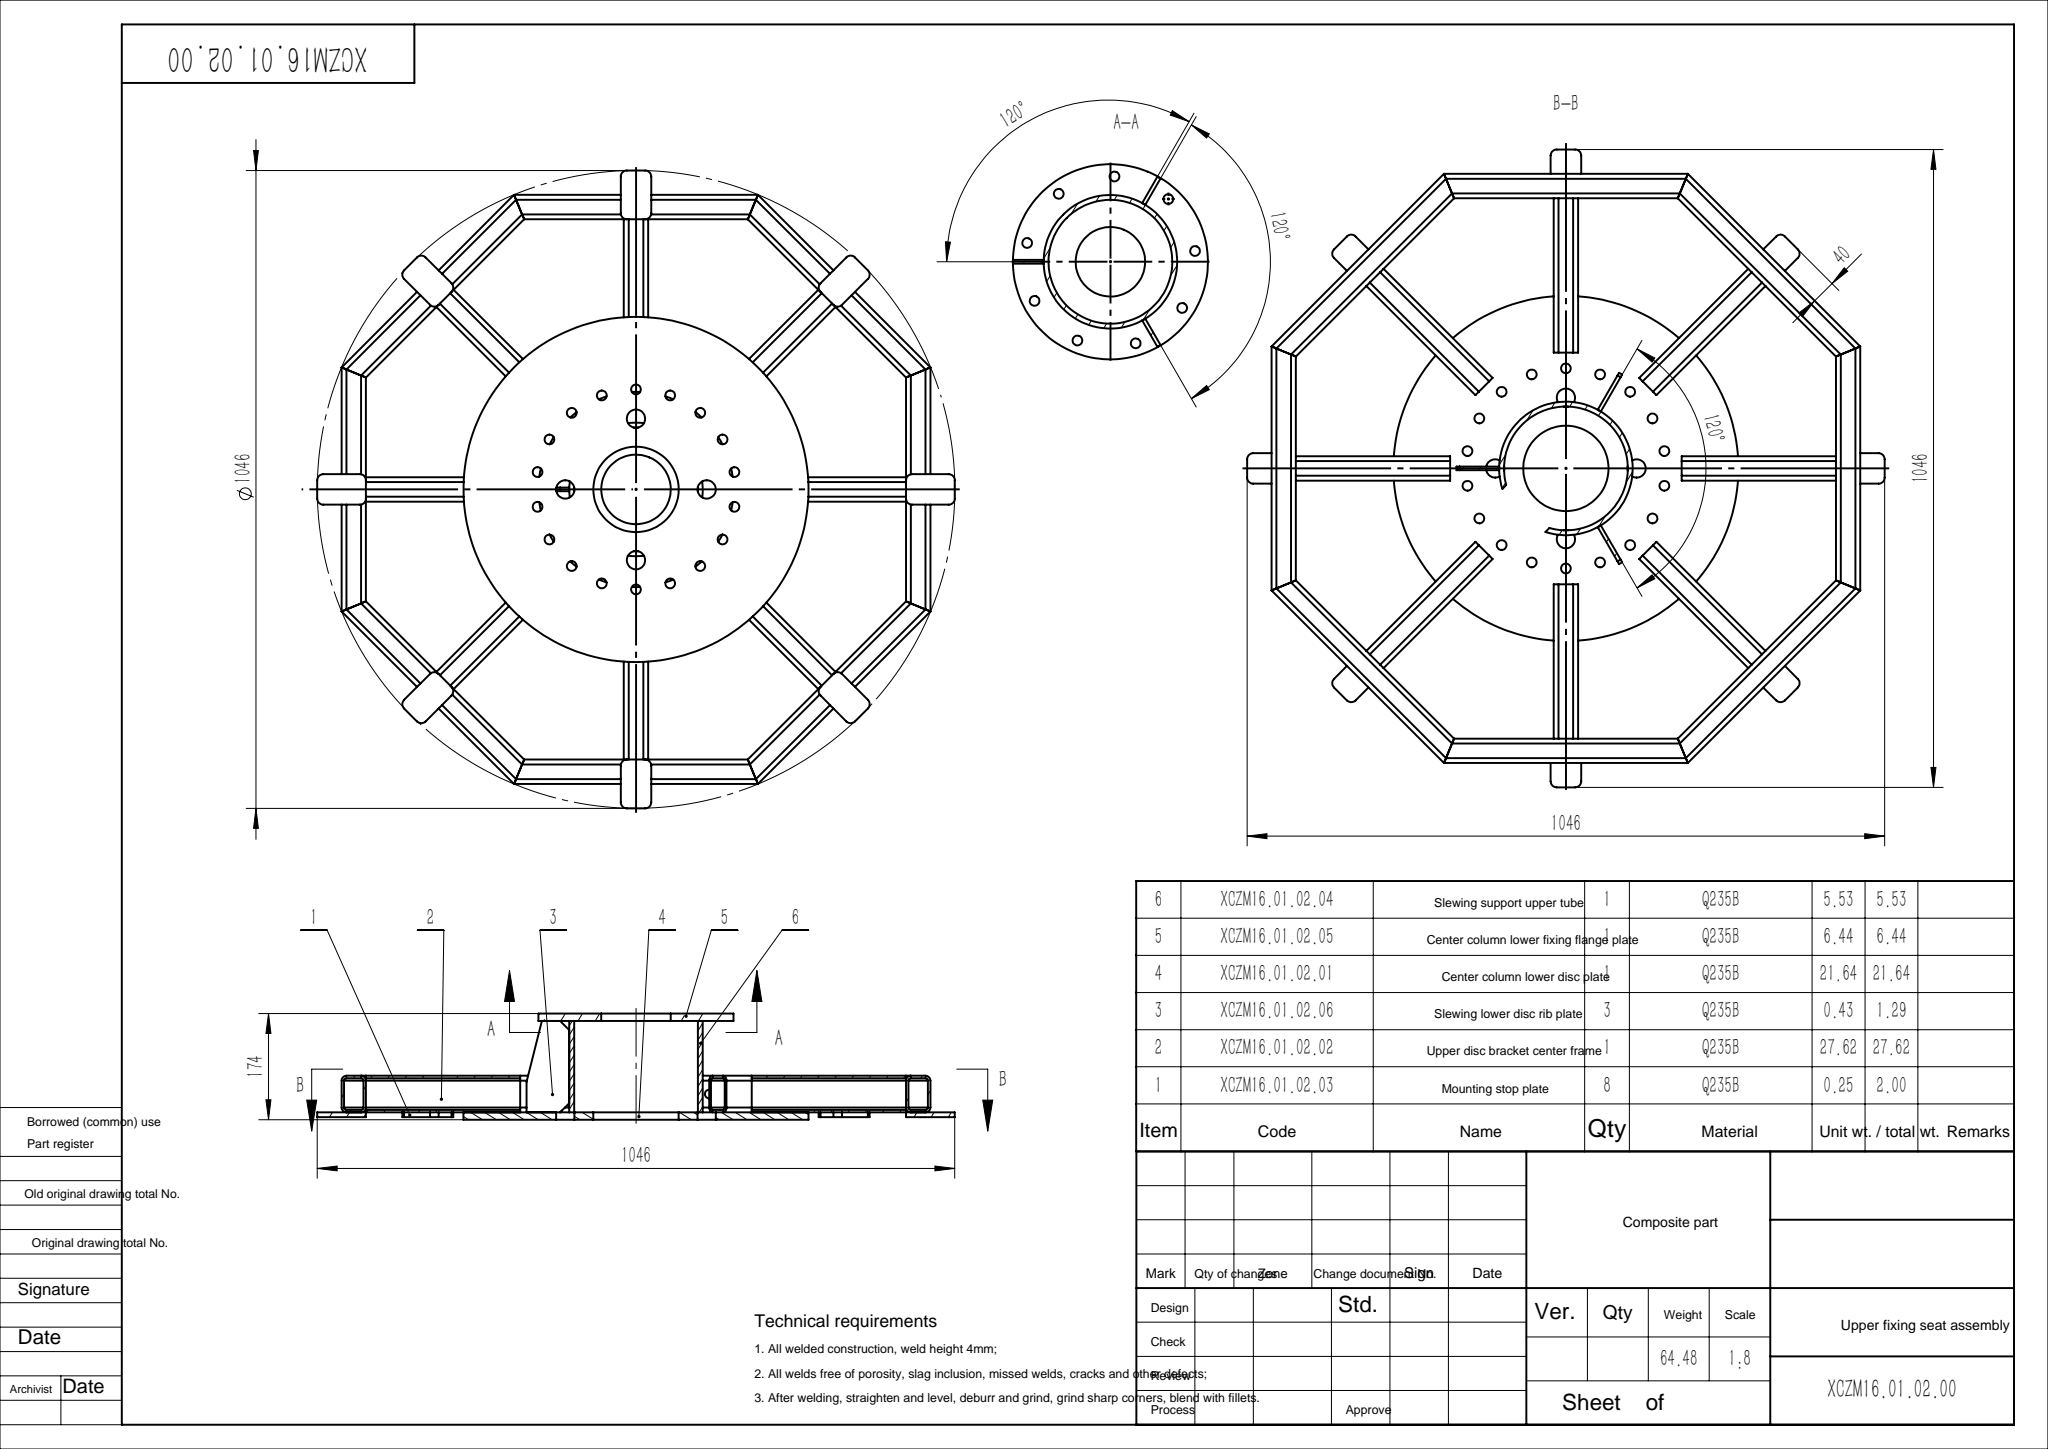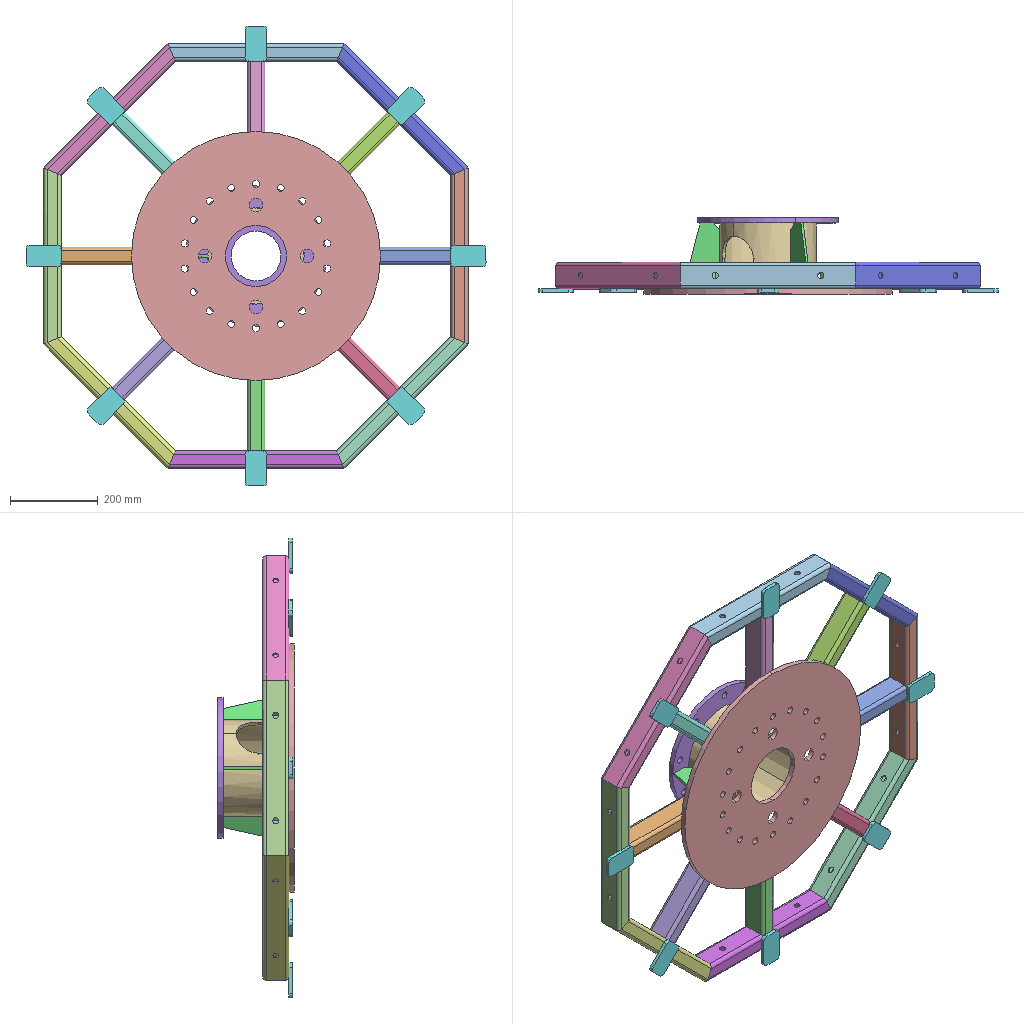Assembly | SolidWorks | 6 different items | 15 placed | box 1046 x 174 x 1046 mm
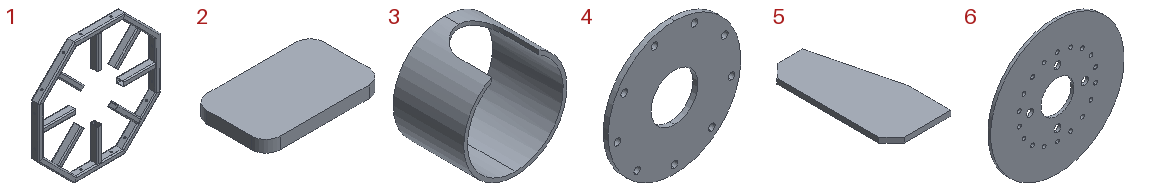Parts list (item | quantity | size | volume | features):
1 | x1 | 966 x 60 x 966 mm | 3518543 mm3 | features WeldCornerFeat 8, CirPattern 2, ICE 1, RefAxis 1, WeldMemberFeat 1, WeldmentFeature 1
2 | x8 | 80 x 50 x 8 mm | 31313 mm3 | features Extrusion 1
3 | x1 | 219 x 150 x 219 mm | 704724 mm3 | features Extrusion 1, ICE 1
4 | x1 | 320 x 12 x 320 mm | 820898 mm3 | features Extrusion 1
5 | x3 | 70 x 150 x 6 mm | 54150 mm3 | features Chamfer 1, Extrusion 1
6 | x1 | 566 x 12 x 566 mm | 2757200 mm3 | features Extrusion 1
Mates (type | each side: item.copy, entity, surface, feature):
Coincident | 1.1 face plane Structural cold-formed hollow rectangular steel (gb t6728-2002) 60×40×4(1) | 6.1 face plane Boss-Extrude1
Coincident | 6.1 plane | assembly plane | 2 times
Concentric | 6.1 face cylinder Boss-Extrude1 | 3.1 face cylinder Boss-Extrude1
Coincident | 6.1 face plane Boss-Extrude1 | 3.1 face plane Boss-Extrude1
Concentric | 3.1 face cylinder Boss-Extrude1 | 4.1 face cylinder Boss-Extrude1
Coincident | 3.1 face plane Boss-Extrude1 | 4.1 face plane Boss-Extrude1
Coincident | 1.1 face plane Structural cold-formed hollow rectangular steel (gb t6728-2002) 60×40×4(1) | 2.1 face plane Boss-Extrude1
Width | 1.1 face plane CirPattern1 | 1.1 face plane CirPattern1 | 2.1 face plane Boss-Extrude1 | 2.1 face plane Boss-Extrude1
DistanceDim | assembly plane | 2.1 face plane Boss-Extrude1
Coincident | 6.1 face plane Boss-Extrude1 | 5.1 face plane Boss-Extrude1
Symmetric | 5.1 face plane Boss-Extrude1 | 5.1 face plane Boss-Extrude1 | assembly plane
Tangent | 3.1 face cylinder Boss-Extrude1 | 5.1 face plane Boss-Extrude1
PlanarAngleDim | 3.1 plane | assembly plane